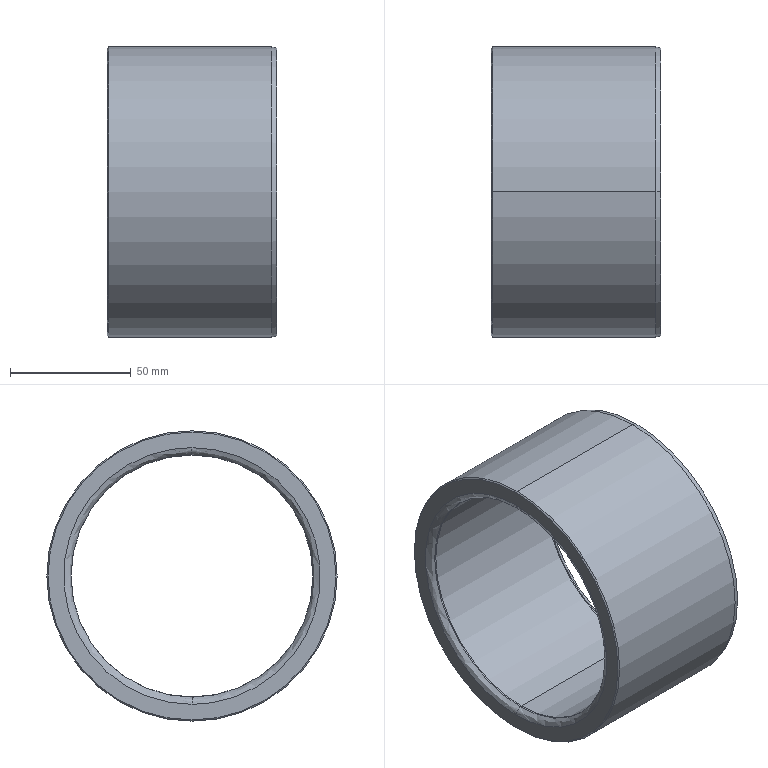Part | SolidWorks | features BaseBody 1 | 1 solid | 18 faces | box 70 x 120 x 120 mm | volume 240473 mm3 | cone 8 | spline 4 | cylinder 4 | plane 2 | commonest cylinder face diameters 100 x2 120 x2
STEP:
#1=CARTESIAN_POINT('',(67.521,-50.092,0.));
#2=VERTEX_POINT('',#1);
#3=CARTESIAN_POINT('',(67.521,0.,50.092));
#4=VERTEX_POINT('',#3);
#5=CARTESIAN_POINT('',(67.521,0.,0.));
#6=DIRECTION('',(-1.,0.,0.));
#7=DIRECTION('',(0.,0.,-1.));
#8=AXIS2_PLACEMENT_3D('',#5,#6,#7);
#9=CIRCLE('',#8,50.092);
#10=EDGE_CURVE('',#2,#4,#9,.T.);
#11=ORIENTED_EDGE('',*,*,#10,.T.);
#12=CARTESIAN_POINT('',(70.,0.,53.046));
#13=VERTEX_POINT('',#12);
#14=CARTESIAN_POINT('',(67.,0.,53.046));
#15=DIRECTION('',(0.,-1.,0.));
#16=DIRECTION('',(0.,0.,1.));
#17=AXIS2_PLACEMENT_3D('',#14,#15,#16);
#18=CIRCLE('',#17,3.);
#19=EDGE_CURVE('',#4,#13,#18,.T.);
#20=ORIENTED_EDGE('',*,*,#19,.T.);
#21=CARTESIAN_POINT('',(70.,0.,-53.046));
#22=VERTEX_POINT('',#21);
#23=CARTESIAN_POINT('',(70.,0.,-53.046));
#24=CARTESIAN_POINT('',(70.,-1.622,-53.046));
#25=CARTESIAN_POINT('',(70.,-4.045,-52.936));
#26=CARTESIAN_POINT('',(70.,-6.855,-52.613));
#27=CARTESIAN_POINT('',(70.,-8.255,-52.403));
#28=CARTESIAN_POINT('',(70.,-8.954,-52.286));
#29=CARTESIAN_POINT('',(70.,-9.303,-52.224));
#30=CARTESIAN_POINT('',(70.,-9.478,-52.193));
#31=CARTESIAN_POINT('',(70.,-9.553,-52.179));
#32=CARTESIAN_POINT('',(70.,-9.603,-52.17));
#33=CARTESIAN_POINT('',(70.,-9.626,-52.166));
#34=CARTESIAN_POINT('',(70.,-11.344,-51.848));
#35=CARTESIAN_POINT('',(70.,-13.847,-51.258));
#36=CARTESIAN_POINT('',(70.,-16.706,-50.36));
#37=CARTESIAN_POINT('',(70.,-18.121,-49.858));
#38=CARTESIAN_POINT('',(70.,-18.825,-49.595));
#39=CARTESIAN_POINT('',(70.,-19.176,-49.459));
#40=CARTESIAN_POINT('',(70.,-19.326,-49.401));
#41=CARTESIAN_POINT('',(70.,-19.426,-49.361));
#42=CARTESIAN_POINT('',(70.,-19.474,-49.342));
#43=CARTESIAN_POINT('',(70.,-21.193,-48.662));
#44=CARTESIAN_POINT('',(70.,-23.63,-47.552));
#45=CARTESIAN_POINT('',(70.,-26.365,-46.046));
#46=CARTESIAN_POINT('',(70.,-27.705,-45.24));
#47=CARTESIAN_POINT('',(70.,-28.369,-44.824));
#48=CARTESIAN_POINT('',(70.,-28.699,-44.613));
#49=CARTESIAN_POINT('',(70.,-28.84,-44.522));
#50=CARTESIAN_POINT('',(70.,-28.934,-44.461));
#51=CARTESIAN_POINT('',(70.,-28.98,-44.431));
#52=CARTESIAN_POINT('',(70.,-32.092,-42.396));
#53=CARTESIAN_POINT('',(70.,-34.92,-40.099));
#54=CARTESIAN_POINT('',(70.,-38.804,-36.215));
#55=CARTESIAN_POINT('',(70.,-40.636,-34.184));
#56=CARTESIAN_POINT('',(70.,-42.582,-31.658));
#57=CARTESIAN_POINT('',(70.,-43.507,-30.356));
#58=CARTESIAN_POINT('',(70.,-43.957,-29.695));
#59=CARTESIAN_POINT('',(70.,-44.179,-29.362));
#60=CARTESIAN_POINT('',(70.,-44.274,-29.219));
#61=CARTESIAN_POINT('',(70.,-44.337,-29.123));
#62=CARTESIAN_POINT('',(70.,-44.369,-29.074));
#63=CARTESIAN_POINT('',(70.,-45.38,-27.527));
#64=CARTESIAN_POINT('',(70.,-46.731,-25.214));
#65=CARTESIAN_POINT('',(70.,-48.097,-22.407));
#66=CARTESIAN_POINT('',(70.,-48.727,-20.975));
#67=CARTESIAN_POINT('',(70.,-49.029,-20.253));
#68=CARTESIAN_POINT('',(70.,-49.176,-19.89));
#69=CARTESIAN_POINT('',(70.,-49.249,-19.708));
#70=CARTESIAN_POINT('',(70.,-49.28,-19.63));
#71=CARTESIAN_POINT('',(70.,-49.301,-19.578));
#72=CARTESIAN_POINT('',(70.,-49.312,-19.551));
#73=CARTESIAN_POINT('',(70.,-49.955,-17.927));
#74=CARTESIAN_POINT('',(70.,-50.785,-15.493));
#75=CARTESIAN_POINT('',(70.,-51.543,-12.593));
#76=CARTESIAN_POINT('',(70.,-51.869,-11.128));
#77=CARTESIAN_POINT('',(70.,-52.019,-10.391));
#78=CARTESIAN_POINT('',(70.,-52.091,-10.022));
#79=CARTESIAN_POINT('',(70.,-52.126,-9.837));
#80=CARTESIAN_POINT('',(70.,-52.141,-9.758));
#81=CARTESIAN_POINT('',(70.,-52.151,-9.705));
#82=CARTESIAN_POINT('',(70.,-52.156,-9.677));
#83=CARTESIAN_POINT('',(70.,-52.751,-6.462));
#84=CARTESIAN_POINT('',(70.,-53.046,-3.244));
#85=CARTESIAN_POINT('',(70.,-53.046,1.622));
#86=CARTESIAN_POINT('',(70.,-52.936,4.045));
#87=CARTESIAN_POINT('',(70.,-52.613,6.855));
#88=CARTESIAN_POINT('',(70.,-52.403,8.255));
#89=CARTESIAN_POINT('',(70.,-52.286,8.954));
#90=CARTESIAN_POINT('',(70.,-52.224,9.303));
#91=CARTESIAN_POINT('',(70.,-52.193,9.478));
#92=CARTESIAN_POINT('',(70.,-52.179,9.553));
#93=CARTESIAN_POINT('',(70.,-52.17,9.603));
#94=CARTESIAN_POINT('',(70.,-52.166,9.626));
#95=CARTESIAN_POINT('',(70.,-51.848,11.344));
#96=CARTESIAN_POINT('',(70.,-51.258,13.847));
#97=CARTESIAN_POINT('',(70.,-50.36,16.706));
#98=CARTESIAN_POINT('',(70.,-49.858,18.121));
#99=CARTESIAN_POINT('',(70.,-49.595,18.825));
#100=CARTESIAN_POINT('',(70.,-49.459,19.176));
#101=CARTESIAN_POINT('',(70.,-49.401,19.326));
#102=CARTESIAN_POINT('',(70.,-49.361,19.426));
#103=CARTESIAN_POINT('',(70.,-49.342,19.474));
#104=CARTESIAN_POINT('',(70.,-48.662,21.193));
#105=CARTESIAN_POINT('',(70.,-47.552,23.63));
#106=CARTESIAN_POINT('',(70.,-46.046,26.365));
#107=CARTESIAN_POINT('',(70.,-45.24,27.705));
#108=CARTESIAN_POINT('',(70.,-44.824,28.369));
#109=CARTESIAN_POINT('',(70.,-44.613,28.699));
#110=CARTESIAN_POINT('',(70.,-44.522,28.84));
#111=CARTESIAN_POINT('',(70.,-44.461,28.934));
#112=CARTESIAN_POINT('',(70.,-44.431,28.98));
#113=CARTESIAN_POINT('',(70.,-42.396,32.092));
#114=CARTESIAN_POINT('',(70.,-40.099,34.92));
#115=CARTESIAN_POINT('',(70.,-36.215,38.804));
#116=CARTESIAN_POINT('',(70.,-34.184,40.636));
#117=CARTESIAN_POINT('',(70.,-31.658,42.582));
#118=CARTESIAN_POINT('',(70.,-30.356,43.507));
#119=CARTESIAN_POINT('',(70.,-29.695,43.957));
#120=CARTESIAN_POINT('',(70.,-29.362,44.179));
#121=CARTESIAN_POINT('',(70.,-29.219,44.274));
#122=CARTESIAN_POINT('',(70.,-29.123,44.337));
#123=CARTESIAN_POINT('',(70.,-29.074,44.369));
#124=CARTESIAN_POINT('',(70.,-27.527,45.38));
#125=CARTESIAN_POINT('',(70.,-25.214,46.731));
#126=CARTESIAN_POINT('',(70.,-22.407,48.097));
#127=CARTESIAN_POINT('',(70.,-20.975,48.727));
#128=CARTESIAN_POINT('',(70.,-20.253,49.029));
#129=CARTESIAN_POINT('',(70.,-19.89,49.176));
#130=CARTESIAN_POINT('',(70.,-19.708,49.249));
#131=CARTESIAN_POINT('',(70.,-19.63,49.28));
#132=CARTESIAN_POINT('',(70.,-19.578,49.301));
#133=CARTESIAN_POINT('',(70.,-19.551,49.312));
#134=CARTESIAN_POINT('',(70.,-17.927,49.955));
#135=CARTESIAN_POINT('',(70.,-15.493,50.785));
#136=CARTESIAN_POINT('',(70.,-12.593,51.543));
#137=CARTESIAN_POINT('',(70.,-11.128,51.869));
#138=CARTESIAN_POINT('',(70.,-10.391,52.019));
#139=CARTESIAN_POINT('',(70.,-10.022,52.091));
#140=CARTESIAN_POINT('',(70.,-9.837,52.126));
#141=CARTESIAN_POINT('',(70.,-9.758,52.141));
#142=CARTESIAN_POINT('',(70.,-9.705,52.151));
#143=CARTESIAN_POINT('',(70.,-9.677,52.156));
#144=CARTESIAN_POINT('',(70.,-6.462,52.751));
#145=CARTESIAN_POINT('',(70.,-3.244,53.046));
#146=CARTESIAN_POINT('',(70.,0.,53.046));
#147=B_SPLINE_CURVE_WITH_KNOTS('',3,(#23,#24,#25,#26,#27,#28,#29,#30,#31,#32,#33,#34,#35,#36,#37,#38,#39,#40,#41,#42,#43,#44,#45,#46,#47,#48,#49,#50,#51,#52,#53,#54,#55,#56,#57,#58,#59,#60,#61,#62,#63,#64,#65,#66,#67,#68,#69,#70,#71,#72,#73,#74,#75,#76,#77,#78,#79,#80,#81,#82,#83,#84,#85,#86,#87,#88,#89,#90,#91,#92,#93,#94,#95,#96,#97,#98,#99,#100,#101,#102,#103,#104,#105,#106,#107,#108,#109,#110,#111,#112,#113,#114,#115,#116,#117,#118,#119,#120,#121,#122,#123,#124,#125,#126,#127,#128,#129,#130,#131,#132,#133,#134,#135,#136,#137,#138,#139,#140,#141,#142,#143,#144,#145,#146),.UNSPECIFIED.,.F.,.F.,(4,1,1,1,1,1,1,2,2,1,1,1,1,1,2,2,1,1,1,1,1,2,2,2,1,1,1,1,1,2,2,1,1,1,1,1,1,2,2,1,1,1,1,1,1,2,2,2,1,1,1,1,1,1,2,2,1,1,1,1,1,2,2,1,1,1,1,1,2,2,2,1,1,1,1,1,2,2,1,1,1,1,1,1,2,2,1,1,1,1,1,1,2,2,4),(0.,0.01562,0.02344,0.02734,0.0293,0.03027,0.03076,0.03101,0.03125,0.04687,0.05469,0.05859,0.06055,0.06152,0.06201,0.0625,0.07812,0.08594,0.08984,0.0918,0.09277,0.09326,0.09375,0.125,0.1406,0.1484,0.1523,0.1543,0.1553,0.1558,0.1562,0.1719,0.1797,0.1836,0.1855,0.1865,0.187,0.1873,0.1875,0.2031,0.2109,0.2148,0.2168,0.2178,0.2183,0.2185,0.2187,0.25,0.2656,0.2734,0.2773,0.2793,0.2803,0.2808,0.281,0.2812,0.2969,0.3047,0.3086,0.3105,0.3115,0.312,0.3125,0.3281,0.3359,0.3398,0.3418,0.3428,0.3433,0.3438,0.375,0.3906,0.3984,0.4023,0.4043,0.4053,0.4058,0.4063,0.4219,0.4297,0.4336,0.4355,0.4365,0.437,0.4373,0.4375,0.4531,0.4609,0.4648,0.4668,0.4678,0.4683,0.4685,0.4688,0.5),.UNSPECIFIED.);
#148=EDGE_CURVE('',#22,#13,#147,.T.);
#149=ORIENTED_EDGE('',*,*,#148,.F.);
#150=CARTESIAN_POINT('',(67.521,0.,-50.092));
#151=VERTEX_POINT('',#150);
#152=CARTESIAN_POINT('',(67.,0.,-53.046));
#153=DIRECTION('',(0.,1.,0.));
#154=DIRECTION('',(0.,0.,-1.));
#155=AXIS2_PLACEMENT_3D('',#152,#153,#154);
#156=CIRCLE('',#155,3.);
#157=EDGE_CURVE('',#151,#22,#156,.T.);
#158=ORIENTED_EDGE('',*,*,#157,.F.);
#159=CARTESIAN_POINT('',(67.521,0.,0.));
#160=DIRECTION('',(-1.,0.,0.));
#161=DIRECTION('',(0.,0.,-1.));
#162=AXIS2_PLACEMENT_3D('',#159,#160,#161);
#163=CIRCLE('',#162,50.092);
#164=EDGE_CURVE('',#151,#2,#163,.T.);
#165=ORIENTED_EDGE('',*,*,#164,.T.);
#166=EDGE_LOOP('',(#11,#20,#149,#158,#165));
#167=FACE_OUTER_BOUND('',#166,.T.);
#168=CARTESIAN_POINT('',(67.521,0.,50.092));
#169=CARTESIAN_POINT('',(67.521,-100.184,50.092));
#170=CARTESIAN_POINT('',(67.521,-100.184,-50.092));
#171=CARTESIAN_POINT('',(67.521,0.,-50.092));
#172=CARTESIAN_POINT('',(69.021,0.,50.356));
#173=CARTESIAN_POINT('',(69.021,-100.713,50.356));
#174=CARTESIAN_POINT('',(69.021,-100.713,-50.356));
#175=CARTESIAN_POINT('',(69.021,0.,-50.356));
#176=CARTESIAN_POINT('',(70.,0.,51.523));
#177=CARTESIAN_POINT('',(70.,-103.046,51.523));
#178=CARTESIAN_POINT('',(70.,-103.046,-51.523));
#179=CARTESIAN_POINT('',(70.,0.,-51.523));
#180=CARTESIAN_POINT('',(70.,0.,53.046));
#181=CARTESIAN_POINT('',(70.,-106.093,53.046));
#182=CARTESIAN_POINT('',(70.,-106.093,-53.046));
#183=CARTESIAN_POINT('',(70.,0.,-53.046));
#184=(BOUNDED_SURFACE()B_SPLINE_SURFACE(3,3,((#168,#169,#170,#171),(#172,#173,#174,#175),(#176,#177,#178,#179),(#180,#181,#182,#183)),.UNSPECIFIED.,.F.,.F.,.F.)B_SPLINE_SURFACE_WITH_KNOTS((4,4),(4,4),(0.,1.),(0.,1.),.UNSPECIFIED.)GEOMETRIC_REPRESENTATION_ITEM()RATIONAL_B_SPLINE_SURFACE(((1.,0.3333,0.3333,1.),(0.844,0.2813,0.2813,0.844),(0.844,0.2813,0.2813,0.844),(1.,0.3333,0.3333,1.)))REPRESENTATION_ITEM('')SURFACE());
#185=ADVANCED_FACE('',(#167),#184,.T.);
#186=CARTESIAN_POINT('',(0.,0.,53.046));
#187=VERTEX_POINT('',#186);
#188=CARTESIAN_POINT('',(0.,0.,-53.046));
#189=VERTEX_POINT('',#188);
#190=CARTESIAN_POINT('',(0.,0.,53.046));
#191=CARTESIAN_POINT('',(0.,-1.622,53.046));
#192=CARTESIAN_POINT('',(0.,-4.045,52.936));
#193=CARTESIAN_POINT('',(0.,-6.855,52.613));
#194=CARTESIAN_POINT('',(0.,-8.255,52.403));
#195=CARTESIAN_POINT('',(0.,-8.954,52.286));
#196=CARTESIAN_POINT('',(0.,-9.303,52.224));
#197=CARTESIAN_POINT('',(0.,-9.478,52.193));
#198=CARTESIAN_POINT('',(0.,-9.553,52.179));
#199=CARTESIAN_POINT('',(0.,-9.603,52.17));
#200=CARTESIAN_POINT('',(0.,-9.626,52.166));
#201=CARTESIAN_POINT('',(0.,-11.344,51.848));
#202=CARTESIAN_POINT('',(0.,-13.847,51.258));
#203=CARTESIAN_POINT('',(0.,-16.706,50.36));
#204=CARTESIAN_POINT('',(0.,-18.121,49.858));
#205=CARTESIAN_POINT('',(0.,-18.825,49.595));
#206=CARTESIAN_POINT('',(0.,-19.176,49.459));
#207=CARTESIAN_POINT('',(0.,-19.326,49.401));
#208=CARTESIAN_POINT('',(0.,-19.426,49.361));
#209=CARTESIAN_POINT('',(0.,-19.474,49.342));
#210=CARTESIAN_POINT('',(0.,-21.193,48.662));
#211=CARTESIAN_POINT('',(0.,-23.63,47.552));
#212=CARTESIAN_POINT('',(0.,-26.365,46.046));
#213=CARTESIAN_POINT('',(0.,-27.705,45.24));
#214=CARTESIAN_POINT('',(0.,-28.369,44.824));
#215=CARTESIAN_POINT('',(0.,-28.699,44.613));
#216=CARTESIAN_POINT('',(0.,-28.84,44.522));
#217=CARTESIAN_POINT('',(0.,-28.934,44.461));
#218=CARTESIAN_POINT('',(0.,-28.98,44.431));
#219=CARTESIAN_POINT('',(0.,-32.092,42.396));
#220=CARTESIAN_POINT('',(0.,-34.92,40.099));
#221=CARTESIAN_POINT('',(0.,-38.804,36.215));
#222=CARTESIAN_POINT('',(0.,-40.636,34.184));
#223=CARTESIAN_POINT('',(0.,-42.582,31.658));
#224=CARTESIAN_POINT('',(0.,-43.507,30.356));
#225=CARTESIAN_POINT('',(0.,-43.957,29.695));
#226=CARTESIAN_POINT('',(0.,-44.179,29.362));
#227=CARTESIAN_POINT('',(0.,-44.274,29.219));
#228=CARTESIAN_POINT('',(0.,-44.337,29.123));
#229=CARTESIAN_POINT('',(0.,-44.369,29.074));
#230=CARTESIAN_POINT('',(0.,-45.38,27.527));
#231=CARTESIAN_POINT('',(0.,-46.731,25.214));
#232=CARTESIAN_POINT('',(0.,-48.097,22.407));
#233=CARTESIAN_POINT('',(0.,-48.727,20.975));
#234=CARTESIAN_POINT('',(0.,-49.029,20.253));
#235=CARTESIAN_POINT('',(0.,-49.176,19.89));
#236=CARTESIAN_POINT('',(0.,-49.249,19.708));
#237=CARTESIAN_POINT('',(0.,-49.28,19.63));
#238=CARTESIAN_POINT('',(0.,-49.301,19.578));
#239=CARTESIAN_POINT('',(0.,-49.312,19.551));
#240=CARTESIAN_POINT('',(0.,-49.955,17.927));
#241=CARTESIAN_POINT('',(0.,-50.785,15.493));
#242=CARTESIAN_POINT('',(0.,-51.543,12.593));
#243=CARTESIAN_POINT('',(0.,-51.869,11.128));
#244=CARTESIAN_POINT('',(0.,-52.019,10.391));
#245=CARTESIAN_POINT('',(0.,-52.091,10.022));
#246=CARTESIAN_POINT('',(0.,-52.126,9.837));
#247=CARTESIAN_POINT('',(0.,-52.141,9.758));
#248=CARTESIAN_POINT('',(0.,-52.151,9.705));
#249=CARTESIAN_POINT('',(0.,-52.156,9.677));
#250=CARTESIAN_POINT('',(0.,-52.751,6.462));
#251=CARTESIAN_POINT('',(0.,-53.046,3.244));
#252=CARTESIAN_POINT('',(0.,-53.046,-1.622));
#253=CARTESIAN_POINT('',(0.,-52.936,-4.045));
#254=CARTESIAN_POINT('',(0.,-52.613,-6.855));
#255=CARTESIAN_POINT('',(0.,-52.403,-8.255));
#256=CARTESIAN_POINT('',(0.,-52.286,-8.954));
#257=CARTESIAN_POINT('',(0.,-52.224,-9.303));
#258=CARTESIAN_POINT('',(0.,-52.193,-9.478));
#259=CARTESIAN_POINT('',(0.,-52.179,-9.553));
#260=CARTESIAN_POINT('',(0.,-52.17,-9.603));
#261=CARTESIAN_POINT('',(0.,-52.166,-9.626));
#262=CARTESIAN_POINT('',(0.,-51.848,-11.344));
#263=CARTESIAN_POINT('',(0.,-51.258,-13.847));
#264=CARTESIAN_POINT('',(0.,-50.36,-16.706));
#265=CARTESIAN_POINT('',(0.,-49.858,-18.121));
#266=CARTESIAN_POINT('',(0.,-49.595,-18.825));
#267=CARTESIAN_POINT('',(0.,-49.459,-19.176));
#268=CARTESIAN_POINT('',(0.,-49.401,-19.326));
#269=CARTESIAN_POINT('',(0.,-49.361,-19.426));
#270=CARTESIAN_POINT('',(0.,-49.342,-19.474));
#271=CARTESIAN_POINT('',(0.,-48.662,-21.193));
#272=CARTESIAN_POINT('',(0.,-47.552,-23.63));
#273=CARTESIAN_POINT('',(0.,-46.046,-26.365));
#274=CARTESIAN_POINT('',(0.,-45.24,-27.705));
#275=CARTESIAN_POINT('',(0.,-44.824,-28.369));
#276=CARTESIAN_POINT('',(0.,-44.613,-28.699));
#277=CARTESIAN_POINT('',(0.,-44.522,-28.84));
#278=CARTESIAN_POINT('',(0.,-44.461,-28.934));
#279=CARTESIAN_POINT('',(0.,-44.431,-28.98));
#280=CARTESIAN_POINT('',(0.,-42.396,-32.092));
#281=CARTESIAN_POINT('',(0.,-40.099,-34.92));
#282=CARTESIAN_POINT('',(0.,-36.215,-38.804));
#283=CARTESIAN_POINT('',(0.,-34.184,-40.636));
#284=CARTESIAN_POINT('',(0.,-31.658,-42.582));
#285=CARTESIAN_POINT('',(0.,-30.356,-43.507));
#286=CARTESIAN_POINT('',(0.,-29.695,-43.957));
#287=CARTESIAN_POINT('',(0.,-29.362,-44.179));
#288=CARTESIAN_POINT('',(0.,-29.219,-44.274));
#289=CARTESIAN_POINT('',(0.,-29.123,-44.337));
#290=CARTESIAN_POINT('',(0.,-29.074,-44.369));
#291=CARTESIAN_POINT('',(0.,-27.527,-45.38));
#292=CARTESIAN_POINT('',(0.,-25.214,-46.731));
#293=CARTESIAN_POINT('',(0.,-22.407,-48.097));
#294=CARTESIAN_POINT('',(0.,-20.975,-48.727));
#295=CARTESIAN_POINT('',(0.,-20.253,-49.029));
#296=CARTESIAN_POINT('',(0.,-19.89,-49.176));
#297=CARTESIAN_POINT('',(0.,-19.708,-49.249));
#298=CARTESIAN_POINT('',(0.,-19.63,-49.28));
#299=CARTESIAN_POINT('',(0.,-19.578,-49.301));
#300=CARTESIAN_POINT('',(0.,-19.551,-49.312));
#301=CARTESIAN_POINT('',(0.,-17.927,-49.955));
#302=CARTESIAN_POINT('',(0.,-15.493,-50.785));
#303=CARTESIAN_POINT('',(0.,-12.593,-51.543));
#304=CARTESIAN_POINT('',(0.,-11.128,-51.869));
#305=CARTESIAN_POINT('',(0.,-10.391,-52.019));
#306=CARTESIAN_POINT('',(0.,-10.022,-52.091));
#307=CARTESIAN_POINT('',(0.,-9.837,-52.126));
#308=CARTESIAN_POINT('',(0.,-9.758,-52.141));
#309=CARTESIAN_POINT('',(0.,-9.705,-52.151));
#310=CARTESIAN_POINT('',(0.,-9.677,-52.156));
#311=CARTESIAN_POINT('',(0.,-6.462,-52.751));
#312=CARTESIAN_POINT('',(0.,-3.245,-53.046));
#313=CARTESIAN_POINT('',(0.,0.,-53.046));
#314=B_SPLINE_CURVE_WITH_KNOTS('',3,(#190,#191,#192,#193,#194,#195,#196,#197,#198,#199,#200,#201,#202,#203,#204,#205,#206,#207,#208,#209,#210,#211,#212,#213,#214,#215,#216,#217,#218,#219,#220,#221,#222,#223,#224,#225,#226,#227,#228,#229,#230,#231,#232,#233,#234,#235,#236,#237,#238,#239,#240,#241,#242,#243,#244,#245,#246,#247,#248,#249,#250,#251,#252,#253,#254,#255,#256,#257,#258,#259,#260,#261,#262,#263,#264,#265,#266,#267,#268,#269,#270,#271,#272,#273,#274,#275,#276,#277,#278,#279,#280,#281,#282,#283,#284,#285,#286,#287,#288,#289,#290,#291,#292,#293,#294,#295,#296,#297,#298,#299,#300,#301,#302,#303,#304,#305,#306,#307,#308,#309,#310,#311,#312,#313),.UNSPECIFIED.,.F.,.F.,(4,1,1,1,1,1,1,2,2,1,1,1,1,1,2,2,1,1,1,1,1,2,2,2,1,1,1,1,1,2,2,1,1,1,1,1,1,2,2,1,1,1,1,1,1,2,2,2,1,1,1,1,1,1,2,2,1,1,1,1,1,2,2,1,1,1,1,1,2,2,2,1,1,1,1,1,2,2,1,1,1,1,1,1,2,2,1,1,1,1,1,1,2,2,4),(0.5,0.5156,0.5234,0.5273,0.5293,0.5303,0.5308,0.531,0.5313,0.5469,0.5547,0.5586,0.5605,0.5615,0.562,0.5625,0.5781,0.5859,0.5898,0.5918,0.5928,0.5933,0.5938,0.625,0.6406,0.6484,0.6523,0.6543,0.6553,0.6558,0.6563,0.6719,0.6797,0.6836,0.6855,0.6865,0.687,0.6873,0.6875,0.7031,0.7109,0.7148,0.7168,0.7178,0.7183,0.7185,0.7187,0.75,0.7656,0.7734,0.7773,0.7793,0.7803,0.7808,0.781,0.7812,0.7969,0.8047,0.8086,0.8105,0.8115,0.812,0.8125,0.8281,0.8359,0.8398,0.8418,0.8428,0.8433,0.8437,0.875,0.8906,0.8984,0.9023,0.9043,0.9053,0.9058,0.9062,0.9219,0.9297,0.9336,0.9355,0.9365,0.937,0.9373,0.9375,0.9531,0.9609,0.9648,0.9668,0.9678,0.9683,0.9685,0.9687,1.),.UNSPECIFIED.);
#315=EDGE_CURVE('',#187,#189,#314,.T.);
#316=ORIENTED_EDGE('',*,*,#315,.F.);
#317=CARTESIAN_POINT('',(2.479,0.,50.092));
#318=VERTEX_POINT('',#317);
#319=CARTESIAN_POINT('',(3.,0.,53.046));
#320=DIRECTION('',(0.,-1.,0.));
#321=DIRECTION('',(0.,0.,1.));
#322=AXIS2_PLACEMENT_3D('',#319,#320,#321);
#323=CIRCLE('',#322,3.);
#324=EDGE_CURVE('',#187,#318,#323,.T.);
#325=ORIENTED_EDGE('',*,*,#324,.T.);
#326=CARTESIAN_POINT('',(2.479,0.,-50.092));
#327=VERTEX_POINT('',#326);
#328=CARTESIAN_POINT('',(2.479,0.,0.));
#329=DIRECTION('',(1.,0.,0.));
#330=DIRECTION('',(0.,0.,-1.));
#331=AXIS2_PLACEMENT_3D('',#328,#329,#330);
#332=CIRCLE('',#331,50.092);
#333=EDGE_CURVE('',#318,#327,#332,.T.);
#334=ORIENTED_EDGE('',*,*,#333,.T.);
#335=CARTESIAN_POINT('',(3.,0.,-53.046));
#336=DIRECTION('',(0.,1.,0.));
#337=DIRECTION('',(0.,0.,-1.));
#338=AXIS2_PLACEMENT_3D('',#335,#336,#337);
#339=CIRCLE('',#338,3.);
#340=EDGE_CURVE('',#189,#327,#339,.T.);
#341=ORIENTED_EDGE('',*,*,#340,.F.);
#342=EDGE_LOOP('',(#316,#325,#334,#341));
#343=FACE_OUTER_BOUND('',#342,.T.);
#344=CARTESIAN_POINT('',(0.,0.,53.046));
#345=CARTESIAN_POINT('',(0.,-106.093,53.046));
#346=CARTESIAN_POINT('',(0.,-106.093,-53.046));
#347=CARTESIAN_POINT('',(0.,0.,-53.046));
#348=CARTESIAN_POINT('',(0.,0.,51.523));
#349=CARTESIAN_POINT('',(0.,-103.046,51.523));
#350=CARTESIAN_POINT('',(0.,-103.046,-51.523));
#351=CARTESIAN_POINT('',(0.,0.,-51.523));
#352=CARTESIAN_POINT('',(0.9791,0.,50.356));
#353=CARTESIAN_POINT('',(0.9791,-100.713,50.356));
#354=CARTESIAN_POINT('',(0.9791,-100.713,-50.356));
#355=CARTESIAN_POINT('',(0.9791,0.,-50.356));
#356=CARTESIAN_POINT('',(2.479,0.,50.092));
#357=CARTESIAN_POINT('',(2.479,-100.184,50.092));
#358=CARTESIAN_POINT('',(2.479,-100.184,-50.092));
#359=CARTESIAN_POINT('',(2.479,0.,-50.092));
#360=(BOUNDED_SURFACE()B_SPLINE_SURFACE(3,3,((#344,#345,#346,#347),(#348,#349,#350,#351),(#352,#353,#354,#355),(#356,#357,#358,#359)),.UNSPECIFIED.,.F.,.F.,.T.)B_SPLINE_SURFACE_WITH_KNOTS((4,4),(4,4),(0.,1.),(0.,1.),.UNSPECIFIED.)GEOMETRIC_REPRESENTATION_ITEM()RATIONAL_B_SPLINE_SURFACE(((1.,0.3333,0.3333,1.),(0.844,0.2813,0.2813,0.844),(0.844,0.2813,0.2813,0.844),(1.,0.3333,0.3333,1.)))REPRESENTATION_ITEM('')SURFACE());
#361=ADVANCED_FACE('',(#343),#360,.T.);
#362=CARTESIAN_POINT('',(68.,0.,60.));
#363=VERTEX_POINT('',#362);
#364=CARTESIAN_POINT('',(68.,0.,-60.));
#365=VERTEX_POINT('',#364);
#366=CARTESIAN_POINT('',(68.,0.,0.));
#367=DIRECTION('',(-1.,0.,0.));
#368=DIRECTION('',(0.,0.,1.));
#369=AXIS2_PLACEMENT_3D('',#366,#367,#368);
#370=CIRCLE('',#369,60.);
#371=EDGE_CURVE('',#363,#365,#370,.T.);
#372=ORIENTED_EDGE('',*,*,#371,.T.);
#373=CARTESIAN_POINT('',(0.5,0.,-60.));
#374=VERTEX_POINT('',#373);
#375=CARTESIAN_POINT('',(70.,0.,-60.));
#376=DIRECTION('',(-1.,0.,0.));
#377=VECTOR('',#376,1000.);
#378=LINE('',#375,#377);
#379=EDGE_CURVE('',#365,#374,#378,.T.);
#380=ORIENTED_EDGE('',*,*,#379,.T.);
#381=CARTESIAN_POINT('',(0.5,0.,60.));
#382=VERTEX_POINT('',#381);
#383=CARTESIAN_POINT('',(0.5,0.,0.));
#384=DIRECTION('',(1.,0.,0.));
#385=DIRECTION('',(0.,0.,1.));
#386=AXIS2_PLACEMENT_3D('',#383,#384,#385);
#387=CIRCLE('',#386,60.);
#388=EDGE_CURVE('',#374,#382,#387,.T.);
#389=ORIENTED_EDGE('',*,*,#388,.T.);
#390=CARTESIAN_POINT('',(70.,0.,60.));
#391=DIRECTION('',(-1.,0.,0.));
#392=VECTOR('',#391,1000.);
#393=LINE('',#390,#392);
#394=EDGE_CURVE('',#363,#382,#393,.T.);
#395=ORIENTED_EDGE('',*,*,#394,.F.);
#396=EDGE_LOOP('',(#372,#380,#389,#395));
#397=FACE_OUTER_BOUND('',#396,.T.);
#398=CARTESIAN_POINT('',(70.,0.,0.));
#399=DIRECTION('',(-1.,0.,0.));
#400=DIRECTION('',(0.,0.,1.));
#401=AXIS2_PLACEMENT_3D('',#398,#399,#400);
#402=CYLINDRICAL_SURFACE('',#401,60.);
#403=ADVANCED_FACE('',(#397),#402,.T.);
#404=CARTESIAN_POINT('',(70.,0.,59.464));
#405=VERTEX_POINT('',#404);
#406=CARTESIAN_POINT('',(70.,0.,-59.464));
#407=VERTEX_POINT('',#406);
#408=CARTESIAN_POINT('',(70.,0.,0.));
#409=DIRECTION('',(-1.,0.,0.));
#410=DIRECTION('',(0.,0.,1.));
#411=AXIS2_PLACEMENT_3D('',#408,#409,#410);
#412=CIRCLE('',#411,59.464);
#413=EDGE_CURVE('',#405,#407,#412,.T.);
#414=ORIENTED_EDGE('',*,*,#413,.T.);
#415=CARTESIAN_POINT('',(68.,0.,-60.));
#416=DIRECTION('',(-0.9659,0.,-0.2588));
#417=VECTOR('',#416,1000.);
#418=LINE('',#415,#417);
#419=EDGE_CURVE('',#407,#365,#418,.T.);
#420=ORIENTED_EDGE('',*,*,#419,.T.);
#421=ORIENTED_EDGE('',*,*,#371,.F.);
#422=CARTESIAN_POINT('',(68.,0.,60.));
#423=DIRECTION('',(-0.9659,0.,0.2588));
#424=VECTOR('',#423,1000.);
#425=LINE('',#422,#424);
#426=EDGE_CURVE('',#405,#363,#425,.T.);
#427=ORIENTED_EDGE('',*,*,#426,.F.);
#428=EDGE_LOOP('',(#414,#420,#421,#427));
#429=FACE_OUTER_BOUND('',#428,.T.);
#430=CARTESIAN_POINT('',(68.,0.,0.));
#431=DIRECTION('',(-1.,0.,0.));
#432=DIRECTION('',(0.,0.,1.));
#433=AXIS2_PLACEMENT_3D('',#430,#431,#432);
#434=CONICAL_SURFACE('',#433,60.,0.2618);
#435=ADVANCED_FACE('',(#429),#434,.T.);
#436=CARTESIAN_POINT('',(0.,0.,-59.5));
#437=VERTEX_POINT('',#436);
#438=CARTESIAN_POINT('',(0.,0.,59.5));
#439=VERTEX_POINT('',#438);
#440=CARTESIAN_POINT('',(0.,0.,0.));
#441=DIRECTION('',(1.,0.,0.));
#442=DIRECTION('',(0.,0.,-1.));
#443=AXIS2_PLACEMENT_3D('',#440,#441,#442);
#444=CIRCLE('',#443,59.5);
#445=EDGE_CURVE('',#437,#439,#444,.T.);
#446=ORIENTED_EDGE('',*,*,#445,.T.);
#447=CARTESIAN_POINT('',(0.5,0.,60.));
#448=DIRECTION('',(0.7071,0.,0.7071));
#449=VECTOR('',#448,1000.);
#450=LINE('',#447,#449);
#451=EDGE_CURVE('',#439,#382,#450,.T.);
#452=ORIENTED_EDGE('',*,*,#451,.T.);
#453=ORIENTED_EDGE('',*,*,#388,.F.);
#454=CARTESIAN_POINT('',(0.5,0.,-60.));
#455=DIRECTION('',(0.7071,0.,-0.7071));
#456=VECTOR('',#455,1000.);
#457=LINE('',#454,#456);
#458=EDGE_CURVE('',#437,#374,#457,.T.);
#459=ORIENTED_EDGE('',*,*,#458,.F.);
#460=EDGE_LOOP('',(#446,#452,#453,#459));
#461=FACE_OUTER_BOUND('',#460,.T.);
#462=CARTESIAN_POINT('',(0.5,0.,0.));
#463=DIRECTION('',(1.,0.,0.));
#464=DIRECTION('',(0.,0.,-1.));
#465=AXIS2_PLACEMENT_3D('',#462,#463,#464);
#466=CONICAL_SURFACE('',#465,60.,0.7854);
#467=ADVANCED_FACE('',(#461),#466,.T.);
#468=CARTESIAN_POINT('',(67.,-50.,0.));
#469=VERTEX_POINT('',#468);
#470=CARTESIAN_POINT('',(67.,0.,-50.));
#471=VERTEX_POINT('',#470);
#472=CARTESIAN_POINT('',(67.,0.,0.));
#473=DIRECTION('',(1.,0.,0.));
#474=DIRECTION('',(0.,0.,-1.));
#475=AXIS2_PLACEMENT_3D('',#472,#473,#474);
#476=CIRCLE('',#475,50.);
#477=EDGE_CURVE('',#469,#471,#476,.T.);
#478=ORIENTED_EDGE('',*,*,#477,.F.);
#479=CARTESIAN_POINT('',(67.521,-50.092,0.));
#480=DIRECTION('',(0.9848,-0.1736,0.));
#481=VECTOR('',#480,1000.);
#482=LINE('',#479,#481);
#483=EDGE_CURVE('',#469,#2,#482,.T.);
#484=ORIENTED_EDGE('',*,*,#483,.T.);
#485=ORIENTED_EDGE('',*,*,#164,.F.);
#486=CARTESIAN_POINT('',(67.521,50.092,0.));
#487=VERTEX_POINT('',#486);
#488=CARTESIAN_POINT('',(67.521,0.,0.));
#489=DIRECTION('',(-1.,0.,0.));
#490=DIRECTION('',(0.,0.,-1.));
#491=AXIS2_PLACEMENT_3D('',#488,#489,#490);
#492=CIRCLE('',#491,50.092);
#493=EDGE_CURVE('',#487,#151,#492,.T.);
#494=ORIENTED_EDGE('',*,*,#493,.F.);
#495=CARTESIAN_POINT('',(67.,50.,0.));
#496=VERTEX_POINT('',#495);
#497=CARTESIAN_POINT('',(67.521,50.092,0.));
#498=DIRECTION('',(0.9848,0.1736,0.));
#499=VECTOR('',#498,1000.);
#500=LINE('',#497,#499);
#501=EDGE_CURVE('',#496,#487,#500,.T.);
#502=ORIENTED_EDGE('',*,*,#501,.F.);
#503=CARTESIAN_POINT('',(67.,0.,0.));
#504=DIRECTION('',(1.,0.,0.));
#505=DIRECTION('',(0.,0.,-1.));
#506=AXIS2_PLACEMENT_3D('',#503,#504,#505);
#507=CIRCLE('',#506,50.);
#508=EDGE_CURVE('',#471,#496,#507,.T.);
#509=ORIENTED_EDGE('',*,*,#508,.F.);
#510=EDGE_LOOP('',(#478,#484,#485,#494,#502,#509));
#511=FACE_OUTER_BOUND('',#510,.T.);
#512=CARTESIAN_POINT('',(67.521,0.,0.));
#513=DIRECTION('',(1.,0.,0.));
#514=DIRECTION('',(0.,1.,0.));
#515=AXIS2_PLACEMENT_3D('',#512,#513,#514);
#516=CONICAL_SURFACE('',#515,50.092,0.1745);
#517=ADVANCED_FACE('',(#511),#516,.F.);
#518=CARTESIAN_POINT('',(3.,0.,-50.));
#519=VERTEX_POINT('',#518);
#520=CARTESIAN_POINT('',(3.,0.,50.));
#521=VERTEX_POINT('',#520);
#522=CARTESIAN_POINT('',(3.,0.,0.));
#523=DIRECTION('',(-1.,0.,0.));
#524=DIRECTION('',(0.,0.,1.));
#525=AXIS2_PLACEMENT_3D('',#522,#523,#524);
#526=CIRCLE('',#525,50.);
#527=EDGE_CURVE('',#519,#521,#526,.T.);
#528=ORIENTED_EDGE('',*,*,#527,.F.);
#529=CARTESIAN_POINT('',(2.479,0.,-50.092));
#530=DIRECTION('',(-0.9848,0.,-0.1736));
#531=VECTOR('',#530,1000.);
#532=LINE('',#529,#531);
#533=EDGE_CURVE('',#519,#327,#532,.T.);
#534=ORIENTED_EDGE('',*,*,#533,.T.);
#535=ORIENTED_EDGE('',*,*,#333,.F.);
#536=CARTESIAN_POINT('',(2.479,0.,50.092));
#537=DIRECTION('',(-0.9848,0.,0.1736));
#538=VECTOR('',#537,1000.);
#539=LINE('',#536,#538);
#540=EDGE_CURVE('',#521,#318,#539,.T.);
#541=ORIENTED_EDGE('',*,*,#540,.F.);
#542=EDGE_LOOP('',(#528,#534,#535,#541));
#543=FACE_OUTER_BOUND('',#542,.T.);
#544=CARTESIAN_POINT('',(2.479,0.,0.));
#545=DIRECTION('',(-1.,0.,0.));
#546=DIRECTION('',(0.,0.,1.));
#547=AXIS2_PLACEMENT_3D('',#544,#545,#546);
#548=CONICAL_SURFACE('',#547,50.092,0.1745);
#549=ADVANCED_FACE('',(#543),#548,.F.);
#550=CARTESIAN_POINT('',(67.,0.,50.));
#551=VERTEX_POINT('',#550);
#552=CARTESIAN_POINT('',(67.,0.,0.));
#553=DIRECTION('',(1.,0.,0.));
#554=DIRECTION('',(0.,0.,-1.));
#555=AXIS2_PLACEMENT_3D('',#552,#553,#554);
#556=CIRCLE('',#555,50.);
#557=EDGE_CURVE('',#551,#469,#556,.T.);
#558=ORIENTED_EDGE('',*,*,#557,.T.);
#559=ORIENTED_EDGE('',*,*,#477,.T.);
#560=CARTESIAN_POINT('',(70.,0.,-50.));
#561=DIRECTION('',(-1.,0.,0.));
#562=VECTOR('',#561,1000.);
#563=LINE('',#560,#562);
#564=EDGE_CURVE('',#471,#519,#563,.T.);
#565=ORIENTED_EDGE('',*,*,#564,.T.);
#566=ORIENTED_EDGE('',*,*,#527,.T.);
#567=CARTESIAN_POINT('',(70.,0.,50.));
#568=DIRECTION('',(-1.,0.,0.));
#569=VECTOR('',#568,1000.);
#570=LINE('',#567,#569);
#571=EDGE_CURVE('',#551,#521,#570,.T.);
#572=ORIENTED_EDGE('',*,*,#571,.F.);
#573=EDGE_LOOP('',(#558,#559,#565,#566,#572));
#574=FACE_OUTER_BOUND('',#573,.T.);
#575=CARTESIAN_POINT('',(70.,0.,0.));
#576=DIRECTION('',(-1.,0.,0.));
#577=DIRECTION('',(0.,0.,1.));
#578=AXIS2_PLACEMENT_3D('',#575,#576,#577);
#579=CYLINDRICAL_SURFACE('',#578,50.);
#580=ADVANCED_FACE('',(#574),#579,.F.);
#581=ORIENTED_EDGE('',*,*,#379,.F.);
#582=CARTESIAN_POINT('',(68.,0.,0.));
#583=DIRECTION('',(-1.,0.,0.));
#584=DIRECTION('',(0.,0.,1.));
#585=AXIS2_PLACEMENT_3D('',#582,#583,#584);
#586=CIRCLE('',#585,60.);
#587=EDGE_CURVE('',#365,#363,#586,.T.);
#588=ORIENTED_EDGE('',*,*,#587,.T.);
#589=ORIENTED_EDGE('',*,*,#394,.T.);
#590=CARTESIAN_POINT('',(0.5,0.,0.));
#591=DIRECTION('',(1.,0.,0.));
#592=DIRECTION('',(0.,0.,1.));
#593=AXIS2_PLACEMENT_3D('',#590,#591,#592);
#594=CIRCLE('',#593,60.);
#595=EDGE_CURVE('',#382,#374,#594,.T.);
#596=ORIENTED_EDGE('',*,*,#595,.T.);
#597=EDGE_LOOP('',(#581,#588,#589,#596));
#598=FACE_OUTER_BOUND('',#597,.T.);
#599=CARTESIAN_POINT('',(70.,0.,0.));
#600=DIRECTION('',(-1.,0.,0.));
#601=DIRECTION('',(0.,0.,1.));
#602=AXIS2_PLACEMENT_3D('',#599,#600,#601);
#603=CYLINDRICAL_SURFACE('',#602,60.);
#604=ADVANCED_FACE('',(#598),#603,.T.);
#605=ORIENTED_EDGE('',*,*,#419,.F.);
#606=CARTESIAN_POINT('',(70.,0.,0.));
#607=DIRECTION('',(-1.,0.,0.));
#608=DIRECTION('',(0.,0.,1.));
#609=AXIS2_PLACEMENT_3D('',#606,#607,#608);
#610=CIRCLE('',#609,59.464);
#611=EDGE_CURVE('',#407,#405,#610,.T.);
#612=ORIENTED_EDGE('',*,*,#611,.T.);
#613=ORIENTED_EDGE('',*,*,#426,.T.);
#614=ORIENTED_EDGE('',*,*,#587,.F.);
#615=EDGE_LOOP('',(#605,#612,#613,#614));
#616=FACE_OUTER_BOUND('',#615,.T.);
#617=CARTESIAN_POINT('',(68.,0.,0.));
#618=DIRECTION('',(-1.,0.,0.));
#619=DIRECTION('',(0.,0.,1.));
#620=AXIS2_PLACEMENT_3D('',#617,#618,#619);
#621=CONICAL_SURFACE('',#620,60.,0.2618);
#622=ADVANCED_FACE('',(#616),#621,.T.);
#623=ORIENTED_EDGE('',*,*,#451,.F.);
#624=CARTESIAN_POINT('',(0.,0.,0.));
#625=DIRECTION('',(1.,0.,0.));
#626=DIRECTION('',(0.,0.,-1.));
#627=AXIS2_PLACEMENT_3D('',#624,#625,#626);
#628=CIRCLE('',#627,59.5);
#629=EDGE_CURVE('',#439,#437,#628,.T.);
#630=ORIENTED_EDGE('',*,*,#629,.T.);
#631=ORIENTED_EDGE('',*,*,#458,.T.);
#632=ORIENTED_EDGE('',*,*,#595,.F.);
#633=EDGE_LOOP('',(#623,#630,#631,#632));
#634=FACE_OUTER_BOUND('',#633,.T.);
#635=CARTESIAN_POINT('',(0.5,0.,0.));
#636=DIRECTION('',(1.,0.,0.));
#637=DIRECTION('',(0.,0.,-1.));
#638=AXIS2_PLACEMENT_3D('',#635,#636,#637);
#639=CONICAL_SURFACE('',#638,60.,0.7854);
#640=ADVANCED_FACE('',(#634),#639,.T.);
#641=ORIENTED_EDGE('',*,*,#148,.T.);
#642=CARTESIAN_POINT('',(70.,0.,53.046));
#643=CARTESIAN_POINT('',(70.,1.622,53.046));
#644=CARTESIAN_POINT('',(70.,4.045,52.936));
#645=CARTESIAN_POINT('',(70.,6.855,52.613));
#646=CARTESIAN_POINT('',(70.,8.255,52.403));
#647=CARTESIAN_POINT('',(70.,8.954,52.286));
#648=CARTESIAN_POINT('',(70.,9.303,52.224));
#649=CARTESIAN_POINT('',(70.,9.478,52.193));
#650=CARTESIAN_POINT('',(70.,9.553,52.179));
#651=CARTESIAN_POINT('',(70.,9.603,52.17));
#652=CARTESIAN_POINT('',(70.,9.626,52.166));
#653=CARTESIAN_POINT('',(70.,11.344,51.848));
#654=CARTESIAN_POINT('',(70.,13.847,51.258));
#655=CARTESIAN_POINT('',(70.,16.706,50.36));
#656=CARTESIAN_POINT('',(70.,18.121,49.858));
#657=CARTESIAN_POINT('',(70.,18.825,49.595));
#658=CARTESIAN_POINT('',(70.,19.176,49.459));
#659=CARTESIAN_POINT('',(70.,19.326,49.401));
#660=CARTESIAN_POINT('',(70.,19.426,49.361));
#661=CARTESIAN_POINT('',(70.,19.474,49.342));
#662=CARTESIAN_POINT('',(70.,21.193,48.662));
#663=CARTESIAN_POINT('',(70.,23.63,47.552));
#664=CARTESIAN_POINT('',(70.,26.365,46.046));
#665=CARTESIAN_POINT('',(70.,27.705,45.24));
#666=CARTESIAN_POINT('',(70.,28.369,44.824));
#667=CARTESIAN_POINT('',(70.,28.699,44.613));
#668=CARTESIAN_POINT('',(70.,28.84,44.522));
#669=CARTESIAN_POINT('',(70.,28.934,44.461));
#670=CARTESIAN_POINT('',(70.,28.98,44.431));
#671=CARTESIAN_POINT('',(70.,32.092,42.396));
#672=CARTESIAN_POINT('',(70.,34.92,40.099));
#673=CARTESIAN_POINT('',(70.,38.804,36.215));
#674=CARTESIAN_POINT('',(70.,40.636,34.184));
#675=CARTESIAN_POINT('',(70.,42.582,31.658));
#676=CARTESIAN_POINT('',(70.,43.507,30.356));
#677=CARTESIAN_POINT('',(70.,43.957,29.695));
#678=CARTESIAN_POINT('',(70.,44.179,29.362));
#679=CARTESIAN_POINT('',(70.,44.274,29.219));
#680=CARTESIAN_POINT('',(70.,44.337,29.123));
#681=CARTESIAN_POINT('',(70.,44.369,29.074));
#682=CARTESIAN_POINT('',(70.,45.38,27.527));
#683=CARTESIAN_POINT('',(70.,46.731,25.214));
#684=CARTESIAN_POINT('',(70.,48.097,22.407));
#685=CARTESIAN_POINT('',(70.,48.727,20.975));
#686=CARTESIAN_POINT('',(70.,49.029,20.253));
#687=CARTESIAN_POINT('',(70.,49.176,19.89));
#688=CARTESIAN_POINT('',(70.,49.249,19.708));
#689=CARTESIAN_POINT('',(70.,49.28,19.63));
#690=CARTESIAN_POINT('',(70.,49.301,19.578));
#691=CARTESIAN_POINT('',(70.,49.312,19.551));
#692=CARTESIAN_POINT('',(70.,49.955,17.927));
#693=CARTESIAN_POINT('',(70.,50.785,15.493));
#694=CARTESIAN_POINT('',(70.,51.543,12.593));
#695=CARTESIAN_POINT('',(70.,51.869,11.128));
#696=CARTESIAN_POINT('',(70.,52.019,10.391));
#697=CARTESIAN_POINT('',(70.,52.091,10.022));
#698=CARTESIAN_POINT('',(70.,52.126,9.837));
#699=CARTESIAN_POINT('',(70.,52.141,9.758));
#700=CARTESIAN_POINT('',(70.,52.151,9.705));
#701=CARTESIAN_POINT('',(70.,52.156,9.677));
#702=CARTESIAN_POINT('',(70.,52.751,6.462));
#703=CARTESIAN_POINT('',(70.,53.046,3.244));
#704=CARTESIAN_POINT('',(70.,53.046,-1.622));
#705=CARTESIAN_POINT('',(70.,52.936,-4.045));
#706=CARTESIAN_POINT('',(70.,52.613,-6.855));
#707=CARTESIAN_POINT('',(70.,52.403,-8.255));
#708=CARTESIAN_POINT('',(70.,52.286,-8.954));
#709=CARTESIAN_POINT('',(70.,52.224,-9.303));
#710=CARTESIAN_POINT('',(70.,52.193,-9.478));
#711=CARTESIAN_POINT('',(70.,52.179,-9.553));
#712=CARTESIAN_POINT('',(70.,52.17,-9.603));
#713=CARTESIAN_POINT('',(70.,52.166,-9.626));
#714=CARTESIAN_POINT('',(70.,51.848,-11.344));
#715=CARTESIAN_POINT('',(70.,51.258,-13.847));
#716=CARTESIAN_POINT('',(70.,50.36,-16.706));
#717=CARTESIAN_POINT('',(70.,49.858,-18.121));
#718=CARTESIAN_POINT('',(70.,49.595,-18.825));
#719=CARTESIAN_POINT('',(70.,49.459,-19.176));
#720=CARTESIAN_POINT('',(70.,49.401,-19.326));
#721=CARTESIAN_POINT('',(70.,49.361,-19.426));
#722=CARTESIAN_POINT('',(70.,49.342,-19.474));
#723=CARTESIAN_POINT('',(70.,48.662,-21.193));
#724=CARTESIAN_POINT('',(70.,47.552,-23.63));
#725=CARTESIAN_POINT('',(70.,46.046,-26.365));
#726=CARTESIAN_POINT('',(70.,45.24,-27.705));
#727=CARTESIAN_POINT('',(70.,44.824,-28.369));
#728=CARTESIAN_POINT('',(70.,44.613,-28.699));
#729=CARTESIAN_POINT('',(70.,44.522,-28.84));
#730=CARTESIAN_POINT('',(70.,44.461,-28.934));
#731=CARTESIAN_POINT('',(70.,44.431,-28.98));
#732=CARTESIAN_POINT('',(70.,42.396,-32.092));
#733=CARTESIAN_POINT('',(70.,40.099,-34.92));
#734=CARTESIAN_POINT('',(70.,36.215,-38.804));
#735=CARTESIAN_POINT('',(70.,34.184,-40.636));
#736=CARTESIAN_POINT('',(70.,31.658,-42.582));
#737=CARTESIAN_POINT('',(70.,30.356,-43.507));
#738=CARTESIAN_POINT('',(70.,29.695,-43.957));
#739=CARTESIAN_POINT('',(70.,29.362,-44.179));
#740=CARTESIAN_POINT('',(70.,29.219,-44.274));
#741=CARTESIAN_POINT('',(70.,29.123,-44.337));
#742=CARTESIAN_POINT('',(70.,29.074,-44.369));
#743=CARTESIAN_POINT('',(70.,27.527,-45.38));
#744=CARTESIAN_POINT('',(70.,25.214,-46.731));
#745=CARTESIAN_POINT('',(70.,22.407,-48.097));
#746=CARTESIAN_POINT('',(70.,20.975,-48.727));
#747=CARTESIAN_POINT('',(70.,20.253,-49.029));
#748=CARTESIAN_POINT('',(70.,19.89,-49.176));
#749=CARTESIAN_POINT('',(70.,19.708,-49.249));
#750=CARTESIAN_POINT('',(70.,19.63,-49.28));
#751=CARTESIAN_POINT('',(70.,19.578,-49.301));
#752=CARTESIAN_POINT('',(70.,19.551,-49.312));
#753=CARTESIAN_POINT('',(70.,17.927,-49.955));
#754=CARTESIAN_POINT('',(70.,15.493,-50.785));
#755=CARTESIAN_POINT('',(70.,12.593,-51.543));
#756=CARTESIAN_POINT('',(70.,11.128,-51.869));
#757=CARTESIAN_POINT('',(70.,10.391,-52.019));
#758=CARTESIAN_POINT('',(70.,10.022,-52.091));
#759=CARTESIAN_POINT('',(70.,9.837,-52.126));
#760=CARTESIAN_POINT('',(70.,9.758,-52.141));
#761=CARTESIAN_POINT('',(70.,9.705,-52.151));
#762=CARTESIAN_POINT('',(70.,9.677,-52.156));
#763=CARTESIAN_POINT('',(70.,6.462,-52.751));
#764=CARTESIAN_POINT('',(70.,3.245,-53.046));
#765=CARTESIAN_POINT('',(70.,0.,-53.046));
#766=B_SPLINE_CURVE_WITH_KNOTS('',3,(#642,#643,#644,#645,#646,#647,#648,#649,#650,#651,#652,#653,#654,#655,#656,#657,#658,#659,#660,#661,#662,#663,#664,#665,#666,#667,#668,#669,#670,#671,#672,#673,#674,#675,#676,#677,#678,#679,#680,#681,#682,#683,#684,#685,#686,#687,#688,#689,#690,#691,#692,#693,#694,#695,#696,#697,#698,#699,#700,#701,#702,#703,#704,#705,#706,#707,#708,#709,#710,#711,#712,#713,#714,#715,#716,#717,#718,#719,#720,#721,#722,#723,#724,#725,#726,#727,#728,#729,#730,#731,#732,#733,#734,#735,#736,#737,#738,#739,#740,#741,#742,#743,#744,#745,#746,#747,#748,#749,#750,#751,#752,#753,#754,#755,#756,#757,#758,#759,#760,#761,#762,#763,#764,#765),.UNSPECIFIED.,.F.,.F.,(4,1,1,1,1,1,1,2,2,1,1,1,1,1,2,2,1,1,1,1,1,2,2,2,1,1,1,1,1,2,2,1,1,1,1,1,1,2,2,1,1,1,1,1,1,2,2,2,1,1,1,1,1,1,2,2,1,1,1,1,1,2,2,1,1,1,1,1,2,2,2,1,1,1,1,1,2,2,1,1,1,1,1,1,2,2,1,1,1,1,1,1,2,2,4),(0.5,0.5156,0.5234,0.5273,0.5293,0.5303,0.5308,0.531,0.5312,0.5469,0.5547,0.5586,0.5605,0.5615,0.562,0.5625,0.5781,0.5859,0.5898,0.5918,0.5928,0.5933,0.5937,0.625,0.6406,0.6484,0.6523,0.6543,0.6553,0.6558,0.6562,0.6719,0.6797,0.6836,0.6855,0.6865,0.687,0.6873,0.6875,0.7031,0.7109,0.7148,0.7168,0.7178,0.7183,0.7185,0.7187,0.75,0.7656,0.7734,0.7773,0.7793,0.7803,0.7808,0.781,0.7812,0.7969,0.8047,0.8086,0.8105,0.8115,0.812,0.8125,0.8281,0.8359,0.8398,0.8418,0.8428,0.8433,0.8437,0.875,0.8906,0.8984,0.9023,0.9043,0.9053,0.9058,0.9062,0.9219,0.9297,0.9336,0.9355,0.9365,0.937,0.9373,0.9375,0.9531,0.9609,0.9648,0.9668,0.9678,0.9683,0.9685,0.9687,1.),.UNSPECIFIED.);
#767=EDGE_CURVE('',#13,#22,#766,.T.);
#768=ORIENTED_EDGE('',*,*,#767,.T.);
#769=EDGE_LOOP('',(#641,#768));
#770=FACE_BOUND('',#769,.T.);
#771=ORIENTED_EDGE('',*,*,#413,.F.);
#772=ORIENTED_EDGE('',*,*,#611,.F.);
#773=EDGE_LOOP('',(#771,#772));
#774=FACE_OUTER_BOUND('',#773,.T.);
#775=CARTESIAN_POINT('',(70.,53.046,0.));
#776=DIRECTION('',(1.,0.,0.));
#777=DIRECTION('',(0.,0.,-1.));
#778=AXIS2_PLACEMENT_3D('',#775,#776,#777);
#779=PLANE('',#778);
#780=ADVANCED_FACE('',(#770,#774),#779,.T.);
#781=ORIENTED_EDGE('',*,*,#445,.F.);
#782=ORIENTED_EDGE('',*,*,#629,.F.);
#783=EDGE_LOOP('',(#781,#782));
#784=FACE_OUTER_BOUND('',#783,.T.);
#785=CARTESIAN_POINT('',(0.,0.,-53.046));
#786=CARTESIAN_POINT('',(0.,1.622,-53.046));
#787=CARTESIAN_POINT('',(0.,4.045,-52.936));
#788=CARTESIAN_POINT('',(0.,6.855,-52.613));
#789=CARTESIAN_POINT('',(0.,8.255,-52.403));
#790=CARTESIAN_POINT('',(0.,8.954,-52.286));
#791=CARTESIAN_POINT('',(0.,9.303,-52.224));
#792=CARTESIAN_POINT('',(0.,9.478,-52.193));
#793=CARTESIAN_POINT('',(0.,9.553,-52.179));
#794=CARTESIAN_POINT('',(0.,9.603,-52.17));
#795=CARTESIAN_POINT('',(0.,9.626,-52.166));
#796=CARTESIAN_POINT('',(0.,11.344,-51.848));
#797=CARTESIAN_POINT('',(0.,13.847,-51.258));
#798=CARTESIAN_POINT('',(0.,16.706,-50.36));
#799=CARTESIAN_POINT('',(0.,18.121,-49.858));
#800=CARTESIAN_POINT('',(0.,18.825,-49.595));
#801=CARTESIAN_POINT('',(0.,19.176,-49.459));
#802=CARTESIAN_POINT('',(0.,19.326,-49.401));
#803=CARTESIAN_POINT('',(0.,19.426,-49.361));
#804=CARTESIAN_POINT('',(0.,19.474,-49.342));
#805=CARTESIAN_POINT('',(0.,21.193,-48.662));
#806=CARTESIAN_POINT('',(0.,23.63,-47.552));
#807=CARTESIAN_POINT('',(0.,26.365,-46.046));
#808=CARTESIAN_POINT('',(0.,27.705,-45.24));
#809=CARTESIAN_POINT('',(0.,28.369,-44.824));
#810=CARTESIAN_POINT('',(0.,28.699,-44.613));
#811=CARTESIAN_POINT('',(0.,28.84,-44.522));
#812=CARTESIAN_POINT('',(0.,28.934,-44.461));
#813=CARTESIAN_POINT('',(0.,28.98,-44.431));
#814=CARTESIAN_POINT('',(0.,32.092,-42.396));
#815=CARTESIAN_POINT('',(0.,34.92,-40.099));
#816=CARTESIAN_POINT('',(0.,38.804,-36.215));
#817=CARTESIAN_POINT('',(0.,40.636,-34.184));
#818=CARTESIAN_POINT('',(0.,42.582,-31.658));
#819=CARTESIAN_POINT('',(0.,43.507,-30.356));
#820=CARTESIAN_POINT('',(0.,43.957,-29.695));
#821=CARTESIAN_POINT('',(0.,44.179,-29.362));
#822=CARTESIAN_POINT('',(0.,44.274,-29.219));
#823=CARTESIAN_POINT('',(0.,44.337,-29.123));
#824=CARTESIAN_POINT('',(0.,44.369,-29.074));
#825=CARTESIAN_POINT('',(0.,45.38,-27.527));
#826=CARTESIAN_POINT('',(0.,46.731,-25.214));
#827=CARTESIAN_POINT('',(0.,48.097,-22.407));
#828=CARTESIAN_POINT('',(0.,48.727,-20.975));
#829=CARTESIAN_POINT('',(0.,49.029,-20.253));
#830=CARTESIAN_POINT('',(0.,49.176,-19.89));
#831=CARTESIAN_POINT('',(0.,49.249,-19.708));
#832=CARTESIAN_POINT('',(0.,49.28,-19.63));
#833=CARTESIAN_POINT('',(0.,49.301,-19.578));
#834=CARTESIAN_POINT('',(0.,49.312,-19.551));
#835=CARTESIAN_POINT('',(0.,49.955,-17.927));
#836=CARTESIAN_POINT('',(0.,50.785,-15.493));
#837=CARTESIAN_POINT('',(0.,51.543,-12.593));
#838=CARTESIAN_POINT('',(0.,51.869,-11.128));
#839=CARTESIAN_POINT('',(0.,52.019,-10.391));
#840=CARTESIAN_POINT('',(0.,52.091,-10.022));
#841=CARTESIAN_POINT('',(0.,52.126,-9.837));
#842=CARTESIAN_POINT('',(0.,52.141,-9.758));
#843=CARTESIAN_POINT('',(0.,52.151,-9.705));
#844=CARTESIAN_POINT('',(0.,52.156,-9.677));
#845=CARTESIAN_POINT('',(0.,52.751,-6.462));
#846=CARTESIAN_POINT('',(0.,53.046,-3.244));
#847=CARTESIAN_POINT('',(0.,53.046,1.622));
#848=CARTESIAN_POINT('',(0.,52.936,4.045));
#849=CARTESIAN_POINT('',(0.,52.613,6.855));
#850=CARTESIAN_POINT('',(0.,52.403,8.255));
#851=CARTESIAN_POINT('',(0.,52.286,8.954));
#852=CARTESIAN_POINT('',(0.,52.224,9.303));
#853=CARTESIAN_POINT('',(0.,52.193,9.478));
#854=CARTESIAN_POINT('',(0.,52.179,9.553));
#855=CARTESIAN_POINT('',(0.,52.17,9.603));
#856=CARTESIAN_POINT('',(0.,52.166,9.626));
#857=CARTESIAN_POINT('',(0.,51.848,11.344));
#858=CARTESIAN_POINT('',(0.,51.258,13.847));
#859=CARTESIAN_POINT('',(0.,50.36,16.706));
#860=CARTESIAN_POINT('',(0.,49.858,18.121));
#861=CARTESIAN_POINT('',(0.,49.595,18.825));
#862=CARTESIAN_POINT('',(0.,49.459,19.176));
#863=CARTESIAN_POINT('',(0.,49.401,19.326));
#864=CARTESIAN_POINT('',(0.,49.361,19.426));
#865=CARTESIAN_POINT('',(0.,49.342,19.474));
#866=CARTESIAN_POINT('',(0.,48.662,21.193));
#867=CARTESIAN_POINT('',(0.,47.552,23.63));
#868=CARTESIAN_POINT('',(0.,46.046,26.365));
#869=CARTESIAN_POINT('',(0.,45.24,27.705));
#870=CARTESIAN_POINT('',(0.,44.824,28.369));
#871=CARTESIAN_POINT('',(0.,44.613,28.699));
#872=CARTESIAN_POINT('',(0.,44.522,28.84));
#873=CARTESIAN_POINT('',(0.,44.461,28.934));
#874=CARTESIAN_POINT('',(0.,44.431,28.98));
#875=CARTESIAN_POINT('',(0.,42.396,32.092));
#876=CARTESIAN_POINT('',(0.,40.099,34.92));
#877=CARTESIAN_POINT('',(0.,36.215,38.804));
#878=CARTESIAN_POINT('',(0.,34.184,40.636));
#879=CARTESIAN_POINT('',(0.,31.658,42.582));
#880=CARTESIAN_POINT('',(0.,30.356,43.507));
#881=CARTESIAN_POINT('',(0.,29.695,43.957));
#882=CARTESIAN_POINT('',(0.,29.362,44.179));
#883=CARTESIAN_POINT('',(0.,29.219,44.274));
#884=CARTESIAN_POINT('',(0.,29.123,44.337));
#885=CARTESIAN_POINT('',(0.,29.074,44.369));
#886=CARTESIAN_POINT('',(0.,27.527,45.38));
#887=CARTESIAN_POINT('',(0.,25.214,46.731));
#888=CARTESIAN_POINT('',(0.,22.407,48.097));
#889=CARTESIAN_POINT('',(0.,20.975,48.727));
#890=CARTESIAN_POINT('',(0.,20.253,49.029));
#891=CARTESIAN_POINT('',(0.,19.89,49.176));
#892=CARTESIAN_POINT('',(0.,19.708,49.249));
#893=CARTESIAN_POINT('',(0.,19.63,49.28));
#894=CARTESIAN_POINT('',(0.,19.578,49.301));
#895=CARTESIAN_POINT('',(0.,19.551,49.312));
#896=CARTESIAN_POINT('',(0.,17.927,49.955));
#897=CARTESIAN_POINT('',(0.,15.493,50.785));
#898=CARTESIAN_POINT('',(0.,12.593,51.543));
#899=CARTESIAN_POINT('',(0.,11.128,51.869));
#900=CARTESIAN_POINT('',(0.,10.391,52.019));
#901=CARTESIAN_POINT('',(0.,10.022,52.091));
#902=CARTESIAN_POINT('',(0.,9.837,52.126));
#903=CARTESIAN_POINT('',(0.,9.758,52.141));
#904=CARTESIAN_POINT('',(0.,9.705,52.151));
#905=CARTESIAN_POINT('',(0.,9.677,52.156));
#906=CARTESIAN_POINT('',(0.,6.462,52.751));
#907=CARTESIAN_POINT('',(0.,3.244,53.046));
#908=CARTESIAN_POINT('',(0.,0.,53.046));
#909=B_SPLINE_CURVE_WITH_KNOTS('',3,(#785,#786,#787,#788,#789,#790,#791,#792,#793,#794,#795,#796,#797,#798,#799,#800,#801,#802,#803,#804,#805,#806,#807,#808,#809,#810,#811,#812,#813,#814,#815,#816,#817,#818,#819,#820,#821,#822,#823,#824,#825,#826,#827,#828,#829,#830,#831,#832,#833,#834,#835,#836,#837,#838,#839,#840,#841,#842,#843,#844,#845,#846,#847,#848,#849,#850,#851,#852,#853,#854,#855,#856,#857,#858,#859,#860,#861,#862,#863,#864,#865,#866,#867,#868,#869,#870,#871,#872,#873,#874,#875,#876,#877,#878,#879,#880,#881,#882,#883,#884,#885,#886,#887,#888,#889,#890,#891,#892,#893,#894,#895,#896,#897,#898,#899,#900,#901,#902,#903,#904,#905,#906,#907,#908),.UNSPECIFIED.,.F.,.F.,(4,1,1,1,1,1,1,2,2,1,1,1,1,1,2,2,1,1,1,1,1,2,2,2,1,1,1,1,1,2,2,1,1,1,1,1,1,2,2,1,1,1,1,1,1,2,2,2,1,1,1,1,1,1,2,2,1,1,1,1,1,2,2,1,1,1,1,1,2,2,2,1,1,1,1,1,2,2,1,1,1,1,1,1,2,2,1,1,1,1,1,1,2,2,4),(0.,0.01562,0.02344,0.02734,0.0293,0.03027,0.03076,0.03101,0.03125,0.04687,0.05469,0.05859,0.06055,0.06152,0.06201,0.0625,0.07812,0.08594,0.08984,0.0918,0.09277,0.09326,0.09375,0.125,0.1406,0.1484,0.1523,0.1543,0.1553,0.1558,0.1563,0.1719,0.1797,0.1836,0.1855,0.1865,0.187,0.1873,0.1875,0.2031,0.2109,0.2148,0.2168,0.2178,0.2183,0.2185,0.2188,0.25,0.2656,0.2734,0.2773,0.2793,0.2803,0.2808,0.281,0.2813,0.2969,0.3047,0.3086,0.3105,0.3115,0.312,0.3125,0.3281,0.3359,0.3398,0.3418,0.3428,0.3433,0.3438,0.375,0.3906,0.3984,0.4023,0.4043,0.4053,0.4058,0.4063,0.4219,0.4297,0.4336,0.4355,0.4365,0.437,0.4373,0.4375,0.4531,0.4609,0.4648,0.4668,0.4678,0.4683,0.4685,0.4688,0.5),.UNSPECIFIED.);
#910=EDGE_CURVE('',#189,#187,#909,.T.);
#911=ORIENTED_EDGE('',*,*,#910,.T.);
#912=ORIENTED_EDGE('',*,*,#315,.T.);
#913=EDGE_LOOP('',(#911,#912));
#914=FACE_BOUND('',#913,.T.);
#915=CARTESIAN_POINT('',(0.,59.5,0.));
#916=DIRECTION('',(-1.,0.,0.));
#917=DIRECTION('',(0.,0.,1.));
#918=AXIS2_PLACEMENT_3D('',#915,#916,#917);
#919=PLANE('',#918);
#920=ADVANCED_FACE('',(#784,#914),#919,.T.);
#921=ORIENTED_EDGE('',*,*,#19,.F.);
#922=CARTESIAN_POINT('',(67.521,0.,0.));
#923=DIRECTION('',(-1.,0.,0.));
#924=DIRECTION('',(0.,0.,-1.));
#925=AXIS2_PLACEMENT_3D('',#922,#923,#924);
#926=CIRCLE('',#925,50.092);
#927=EDGE_CURVE('',#4,#487,#926,.T.);
#928=ORIENTED_EDGE('',*,*,#927,.T.);
#929=ORIENTED_EDGE('',*,*,#493,.T.);
#930=ORIENTED_EDGE('',*,*,#157,.T.);
#931=ORIENTED_EDGE('',*,*,#767,.F.);
#932=EDGE_LOOP('',(#921,#928,#929,#930,#931));
#933=FACE_OUTER_BOUND('',#932,.T.);
#934=CARTESIAN_POINT('',(67.521,0.,-50.092));
#935=CARTESIAN_POINT('',(67.521,100.184,-50.092));
#936=CARTESIAN_POINT('',(67.521,100.184,50.092));
#937=CARTESIAN_POINT('',(67.521,0.,50.092));
#938=CARTESIAN_POINT('',(69.021,0.,-50.356));
#939=CARTESIAN_POINT('',(69.021,100.713,-50.356));
#940=CARTESIAN_POINT('',(69.021,100.713,50.356));
#941=CARTESIAN_POINT('',(69.021,0.,50.356));
#942=CARTESIAN_POINT('',(70.,0.,-51.523));
#943=CARTESIAN_POINT('',(70.,103.046,-51.523));
#944=CARTESIAN_POINT('',(70.,103.046,51.523));
#945=CARTESIAN_POINT('',(70.,0.,51.523));
#946=CARTESIAN_POINT('',(70.,0.,-53.046));
#947=CARTESIAN_POINT('',(70.,106.093,-53.046));
#948=CARTESIAN_POINT('',(70.,106.093,53.046));
#949=CARTESIAN_POINT('',(70.,0.,53.046));
#950=(BOUNDED_SURFACE()B_SPLINE_SURFACE(3,3,((#934,#935,#936,#937),(#938,#939,#940,#941),(#942,#943,#944,#945),(#946,#947,#948,#949)),.UNSPECIFIED.,.F.,.F.,.T.)B_SPLINE_SURFACE_WITH_KNOTS((4,4),(4,4),(0.,1.),(0.,1.),.UNSPECIFIED.)GEOMETRIC_REPRESENTATION_ITEM()RATIONAL_B_SPLINE_SURFACE(((1.,0.3333,0.3333,1.),(0.844,0.2813,0.2813,0.844),(0.844,0.2813,0.2813,0.844),(1.,0.3333,0.3333,1.)))REPRESENTATION_ITEM('')SURFACE());
#951=ADVANCED_FACE('',(#933),#950,.T.);
#952=ORIENTED_EDGE('',*,*,#324,.F.);
#953=ORIENTED_EDGE('',*,*,#910,.F.);
#954=ORIENTED_EDGE('',*,*,#340,.T.);
#955=CARTESIAN_POINT('',(2.479,0.,0.));
#956=DIRECTION('',(1.,0.,0.));
#957=DIRECTION('',(0.,0.,-1.));
#958=AXIS2_PLACEMENT_3D('',#955,#956,#957);
#959=CIRCLE('',#958,50.092);
#960=EDGE_CURVE('',#327,#318,#959,.T.);
#961=ORIENTED_EDGE('',*,*,#960,.T.);
#962=EDGE_LOOP('',(#952,#953,#954,#961));
#963=FACE_OUTER_BOUND('',#962,.T.);
#964=CARTESIAN_POINT('',(0.,0.,-53.046));
#965=CARTESIAN_POINT('',(0.,106.093,-53.046));
#966=CARTESIAN_POINT('',(0.,106.093,53.046));
#967=CARTESIAN_POINT('',(0.,0.,53.046));
#968=CARTESIAN_POINT('',(0.,0.,-51.523));
#969=CARTESIAN_POINT('',(0.,103.046,-51.523));
#970=CARTESIAN_POINT('',(0.,103.046,51.523));
#971=CARTESIAN_POINT('',(0.,0.,51.523));
#972=CARTESIAN_POINT('',(0.9791,0.,-50.356));
#973=CARTESIAN_POINT('',(0.9791,100.713,-50.356));
#974=CARTESIAN_POINT('',(0.9791,100.713,50.356));
#975=CARTESIAN_POINT('',(0.9791,0.,50.356));
#976=CARTESIAN_POINT('',(2.479,0.,-50.092));
#977=CARTESIAN_POINT('',(2.479,100.184,-50.092));
#978=CARTESIAN_POINT('',(2.479,100.184,50.092));
#979=CARTESIAN_POINT('',(2.479,0.,50.092));
#980=(BOUNDED_SURFACE()B_SPLINE_SURFACE(3,3,((#964,#965,#966,#967),(#968,#969,#970,#971),(#972,#973,#974,#975),(#976,#977,#978,#979)),.UNSPECIFIED.,.F.,.F.,.F.)B_SPLINE_SURFACE_WITH_KNOTS((4,4),(4,4),(0.,1.),(0.,1.),.UNSPECIFIED.)GEOMETRIC_REPRESENTATION_ITEM()RATIONAL_B_SPLINE_SURFACE(((1.,0.3333,0.3333,1.),(0.844,0.2813,0.2813,0.844),(0.844,0.2813,0.2813,0.844),(1.,0.3333,0.3333,1.)))REPRESENTATION_ITEM('')SURFACE());
#981=ADVANCED_FACE('',(#963),#980,.T.);
#982=ORIENTED_EDGE('',*,*,#483,.F.);
#983=ORIENTED_EDGE('',*,*,#557,.F.);
#984=CARTESIAN_POINT('',(67.,0.,0.));
#985=DIRECTION('',(1.,0.,0.));
#986=DIRECTION('',(0.,0.,-1.));
#987=AXIS2_PLACEMENT_3D('',#984,#985,#986);
#988=CIRCLE('',#987,50.);
#989=EDGE_CURVE('',#496,#551,#988,.T.);
#990=ORIENTED_EDGE('',*,*,#989,.F.);
#991=ORIENTED_EDGE('',*,*,#501,.T.);
#992=ORIENTED_EDGE('',*,*,#927,.F.);
#993=ORIENTED_EDGE('',*,*,#10,.F.);
#994=EDGE_LOOP('',(#982,#983,#990,#991,#992,#993));
#995=FACE_OUTER_BOUND('',#994,.T.);
#996=CARTESIAN_POINT('',(67.521,0.,0.));
#997=DIRECTION('',(1.,0.,0.));
#998=DIRECTION('',(0.,1.,0.));
#999=AXIS2_PLACEMENT_3D('',#996,#997,#998);
#1000=CONICAL_SURFACE('',#999,50.092,0.1745);
#1001=ADVANCED_FACE('',(#995),#1000,.F.);
#1002=ORIENTED_EDGE('',*,*,#533,.F.);
#1003=CARTESIAN_POINT('',(3.,0.,0.));
#1004=DIRECTION('',(-1.,0.,0.));
#1005=DIRECTION('',(0.,0.,1.));
#1006=AXIS2_PLACEMENT_3D('',#1003,#1004,#1005);
#1007=CIRCLE('',#1006,50.);
#1008=EDGE_CURVE('',#521,#519,#1007,.T.);
#1009=ORIENTED_EDGE('',*,*,#1008,.F.);
#1010=ORIENTED_EDGE('',*,*,#540,.T.);
#1011=ORIENTED_EDGE('',*,*,#960,.F.);
#1012=EDGE_LOOP('',(#1002,#1009,#1010,#1011));
#1013=FACE_OUTER_BOUND('',#1012,.T.);
#1014=CARTESIAN_POINT('',(2.479,0.,0.));
#1015=DIRECTION('',(-1.,0.,0.));
#1016=DIRECTION('',(0.,0.,1.));
#1017=AXIS2_PLACEMENT_3D('',#1014,#1015,#1016);
#1018=CONICAL_SURFACE('',#1017,50.092,0.1745);
#1019=ADVANCED_FACE('',(#1013),#1018,.F.);
#1020=ORIENTED_EDGE('',*,*,#564,.F.);
#1021=ORIENTED_EDGE('',*,*,#508,.T.);
#1022=ORIENTED_EDGE('',*,*,#989,.T.);
#1023=ORIENTED_EDGE('',*,*,#571,.T.);
#1024=ORIENTED_EDGE('',*,*,#1008,.T.);
#1025=EDGE_LOOP('',(#1020,#1021,#1022,#1023,#1024));
#1026=FACE_OUTER_BOUND('',#1025,.T.);
#1027=CARTESIAN_POINT('',(70.,0.,0.));
#1028=DIRECTION('',(-1.,0.,0.));
#1029=DIRECTION('',(0.,0.,1.));
#1030=AXIS2_PLACEMENT_3D('',#1027,#1028,#1029);
#1031=CYLINDRICAL_SURFACE('',#1030,50.);
#1032=ADVANCED_FACE('',(#1026),#1031,.F.);
#1033=CLOSED_SHELL('',(#185,#361,#403,#435,#467,#517,#549,#580,#604,#622,#640,#780,#920,#951,#981,#1001,#1019,#1032));
#1034=MANIFOLD_SOLID_BREP('',#1033);
#1035=CARTESIAN_POINT('',(0.,0.,0.));
#1036=DIRECTION('',(0.,0.,1.));
#1037=DIRECTION('',(1.,0.,0.));
#1038=AXIS2_PLACEMENT_3D('',#1035,#1036,#1037);
#1039=(LENGTH_UNIT()NAMED_UNIT(*)SI_UNIT(.MILLI.,.METRE.));
#1040=UNCERTAINTY_MEASURE_WITH_UNIT(LENGTH_MEASURE(0.00001),#1039,'','');
#1041=(NAMED_UNIT(*)PLANE_ANGLE_UNIT()SI_UNIT($,.RADIAN.));
#1042=(NAMED_UNIT(*)SI_UNIT($,.STERADIAN.)SOLID_ANGLE_UNIT());
#1043=(GEOMETRIC_REPRESENTATION_CONTEXT(3)GLOBAL_UNCERTAINTY_ASSIGNED_CONTEXT((#1040))GLOBAL_UNIT_ASSIGNED_CONTEXT((#1039,#1041,#1042))REPRESENTATION_CONTEXT('',''));
#1044=ADVANCED_BREP_SHAPE_REPRESENTATION('',(#1034,#1038),#1043);